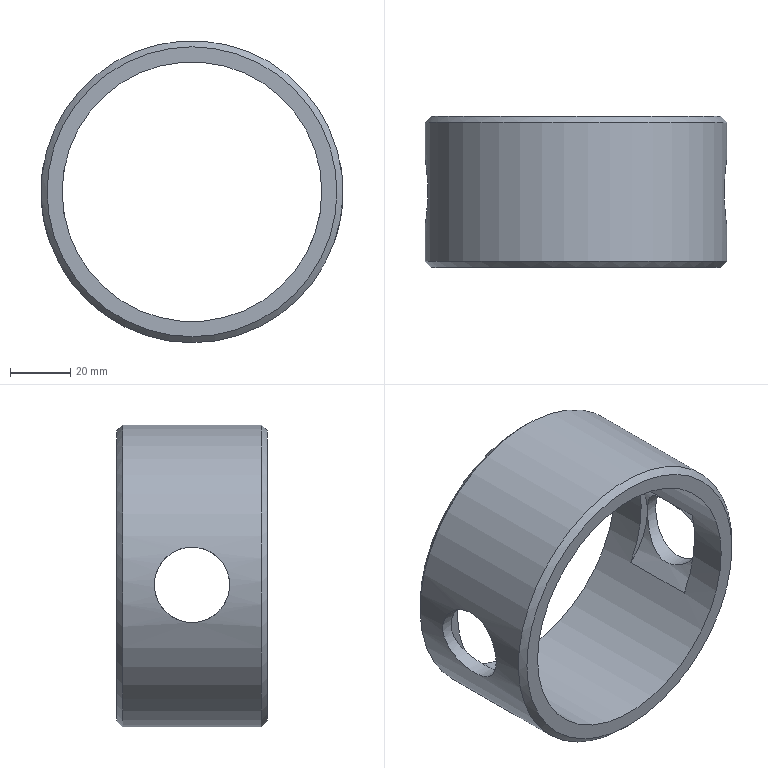Part | NX | features DATUM_CSYS 6, EXTRUDE 5, SKETCH 5, EXTRACT_DATUM_AXIS 4, EXTRACT_DATUM_PLANE 4, EXTRACT_STRING 4, CHAMFER 1, Instance Feature 1, Mirror Feature 1 | 1 solid | 16 faces | box 100.002 x 50 x 100 mm | volume 93333 mm3 | cylinder 8 | plane 6 | cone 2 | commonest cylinder face diameters 44 x4 25 x2 86 x1 100 x1
STEP:
#1=CARTESIAN_POINT('',(-41.856,-12.5,9.851));
#2=VERTEX_POINT('',#1);
#3=CARTESIAN_POINT('',(-46.,-12.5,-3.));
#4=VERTEX_POINT('',#3);
#5=CARTESIAN_POINT('',(-24.,-12.5,-3.));
#6=DIRECTION('',(0.,1.,0.));
#7=DIRECTION('',(-1.,0.,0.));
#8=AXIS2_PLACEMENT_3D('',#5,#6,#7);
#9=CIRCLE('',#8,22.);
#10=EDGE_CURVE('',#2,#4,#9,.F.);
#11=ORIENTED_EDGE('',*,*,#10,.T.);
#12=CARTESIAN_POINT('',(-46.,12.5,-3.));
#13=VERTEX_POINT('',#12);
#14=CARTESIAN_POINT('',(-46.,-12.5,-3.));
#15=CARTESIAN_POINT('',(-46.,-12.5,-1.308));
#16=CARTESIAN_POINT('',(-45.595,-11.807,2.009));
#17=CARTESIAN_POINT('',(-44.159,-9.032,6.076));
#18=CARTESIAN_POINT('',(-42.612,-5.019,8.799));
#19=CARTESIAN_POINT('',(-41.851,-0.003334,9.849));
#20=CARTESIAN_POINT('',(-42.609,5.011,8.804));
#21=CARTESIAN_POINT('',(-44.164,9.044,6.066));
#22=CARTESIAN_POINT('',(-45.595,11.806,2.005));
#23=CARTESIAN_POINT('',(-46.,12.5,-1.306));
#24=CARTESIAN_POINT('',(-46.,12.5,-3.));
#25=B_SPLINE_CURVE_WITH_KNOTS('',3,(#14,#15,#16,#17,#18,#19,#20,#21,#22,#23,#24),.UNSPECIFIED.,.F.,.F.,(4,1,1,1,1,1,1,1,4),(0.,0.004998,0.009995,0.01499,0.01999,0.02499,0.02999,0.03498,0.03998),.UNSPECIFIED.);
#26=EDGE_CURVE('',#13,#4,#25,.F.);
#27=ORIENTED_EDGE('',*,*,#26,.F.);
#28=CARTESIAN_POINT('',(-41.856,12.5,9.851));
#29=VERTEX_POINT('',#28);
#30=CARTESIAN_POINT('',(-24.,12.5,-3.));
#31=DIRECTION('',(0.,1.,0.));
#32=DIRECTION('',(-1.,0.,0.));
#33=AXIS2_PLACEMENT_3D('',#30,#31,#32);
#34=CIRCLE('',#33,22.);
#35=EDGE_CURVE('',#29,#13,#34,.F.);
#36=ORIENTED_EDGE('',*,*,#35,.F.);
#37=CARTESIAN_POINT('',(-41.856,0.,9.851));
#38=DIRECTION('',(0.,1.,0.));
#39=VECTOR('',#38,1000.);
#40=LINE('',#37,#39);
#41=EDGE_CURVE('',#29,#2,#40,.F.);
#42=ORIENTED_EDGE('',*,*,#41,.T.);
#43=EDGE_LOOP('',(#11,#27,#36,#42));
#44=FACE_BOUND('',#43,.T.);
#45=CARTESIAN_POINT('',(-24.,-12.5,-3.));
#46=DIRECTION('',(0.,1.,0.));
#47=DIRECTION('',(0.,0.,1.));
#48=AXIS2_PLACEMENT_3D('',#45,#46,#47);
#49=CYLINDRICAL_SURFACE('',#48,22.);
#50=ADVANCED_FACE('',(#44),#49,.F.);
#51=CARTESIAN_POINT('',(38.144,-12.5,-19.851));
#52=VERTEX_POINT('',#51);
#53=CARTESIAN_POINT('',(41.856,-12.5,9.851));
#54=VERTEX_POINT('',#53);
#55=CARTESIAN_POINT('',(0.,-12.5,0.));
#56=DIRECTION('',(0.,-1.,0.));
#57=DIRECTION('',(0.,0.,-1.));
#58=AXIS2_PLACEMENT_3D('',#55,#56,#57);
#59=CIRCLE('',#58,43.);
#60=EDGE_CURVE('',#52,#54,#59,.T.);
#61=ORIENTED_EDGE('',*,*,#60,.F.);
#62=CARTESIAN_POINT('',(38.144,12.5,-19.851));
#63=VERTEX_POINT('',#62);
#64=CARTESIAN_POINT('',(38.144,0.,-19.851));
#65=DIRECTION('',(0.,1.,0.));
#66=VECTOR('',#65,1000.);
#67=LINE('',#64,#66);
#68=EDGE_CURVE('',#52,#63,#67,.T.);
#69=ORIENTED_EDGE('',*,*,#68,.T.);
#70=CARTESIAN_POINT('',(41.856,12.5,9.851));
#71=VERTEX_POINT('',#70);
#72=CARTESIAN_POINT('',(0.,12.5,0.));
#73=DIRECTION('',(0.,-1.,0.));
#74=DIRECTION('',(0.,0.,-1.));
#75=AXIS2_PLACEMENT_3D('',#72,#73,#74);
#76=CIRCLE('',#75,43.);
#77=EDGE_CURVE('',#63,#71,#76,.T.);
#78=ORIENTED_EDGE('',*,*,#77,.T.);
#79=CARTESIAN_POINT('',(41.856,0.,9.851));
#80=DIRECTION('',(0.,1.,0.));
#81=VECTOR('',#80,1000.);
#82=LINE('',#79,#81);
#83=EDGE_CURVE('',#71,#54,#82,.F.);
#84=ORIENTED_EDGE('',*,*,#83,.T.);
#85=EDGE_LOOP('',(#61,#69,#78,#84));
#86=FACE_BOUND('',#85,.T.);
#87=CARTESIAN_POINT('',(43.,-25.,0.));
#88=VERTEX_POINT('',#87);
#89=CARTESIAN_POINT('',(0.,-25.,0.));
#90=DIRECTION('',(0.,-1.,0.));
#91=DIRECTION('',(1.,0.,0.));
#92=AXIS2_PLACEMENT_3D('',#89,#90,#91);
#93=CIRCLE('',#92,43.);
#94=EDGE_CURVE('',#88,#88,#93,.T.);
#95=ORIENTED_EDGE('',*,*,#94,.T.);
#96=EDGE_LOOP('',(#95));
#97=FACE_BOUND('',#96,.T.);
#98=CARTESIAN_POINT('',(43.,25.,0.));
#99=VERTEX_POINT('',#98);
#100=CARTESIAN_POINT('',(0.,25.,0.));
#101=DIRECTION('',(0.,-1.,0.));
#102=DIRECTION('',(1.,0.,0.));
#103=AXIS2_PLACEMENT_3D('',#100,#101,#102);
#104=CIRCLE('',#103,43.);
#105=EDGE_CURVE('',#99,#99,#104,.T.);
#106=ORIENTED_EDGE('',*,*,#105,.F.);
#107=EDGE_LOOP('',(#106));
#108=FACE_BOUND('',#107,.T.);
#109=CARTESIAN_POINT('',(-38.144,-12.5,-19.851));
#110=VERTEX_POINT('',#109);
#111=CARTESIAN_POINT('',(-38.144,12.5,-19.851));
#112=VERTEX_POINT('',#111);
#113=CARTESIAN_POINT('',(-38.144,0.,-19.851));
#114=DIRECTION('',(0.,1.,0.));
#115=VECTOR('',#114,1000.);
#116=LINE('',#113,#115);
#117=EDGE_CURVE('',#110,#112,#116,.T.);
#118=ORIENTED_EDGE('',*,*,#117,.F.);
#119=CARTESIAN_POINT('',(0.,-12.5,0.));
#120=DIRECTION('',(0.,1.,0.));
#121=DIRECTION('',(0.,0.,1.));
#122=AXIS2_PLACEMENT_3D('',#119,#120,#121);
#123=CIRCLE('',#122,43.);
#124=EDGE_CURVE('',#110,#2,#123,.T.);
#125=ORIENTED_EDGE('',*,*,#124,.T.);
#126=ORIENTED_EDGE('',*,*,#41,.F.);
#127=CARTESIAN_POINT('',(0.,12.5,0.));
#128=DIRECTION('',(0.,1.,0.));
#129=DIRECTION('',(0.,0.,1.));
#130=AXIS2_PLACEMENT_3D('',#127,#128,#129);
#131=CIRCLE('',#130,43.);
#132=EDGE_CURVE('',#112,#29,#131,.T.);
#133=ORIENTED_EDGE('',*,*,#132,.F.);
#134=EDGE_LOOP('',(#118,#125,#126,#133));
#135=FACE_BOUND('',#134,.T.);
#136=CARTESIAN_POINT('',(0.,-25.,0.));
#137=DIRECTION('',(0.,1.,0.));
#138=DIRECTION('',(0.,0.,1.));
#139=AXIS2_PLACEMENT_3D('',#136,#137,#138);
#140=CYLINDRICAL_SURFACE('',#139,43.);
#141=ADVANCED_FACE('',(#86,#97,#108,#135),#140,.F.);
#142=CARTESIAN_POINT('',(-47.537,0.,-15.5));
#143=VERTEX_POINT('',#142);
#144=CARTESIAN_POINT('',(-47.76,-4.945,-14.831));
#145=CARTESIAN_POINT('',(-47.426,0.003336,-15.833));
#146=CARTESIAN_POINT('',(-47.759,4.932,-14.835));
#147=CARTESIAN_POINT('',(-48.841,10.436,-11.16));
#148=CARTESIAN_POINT('',(-49.982,13.155,-4.738));
#149=CARTESIAN_POINT('',(-50.038,11.869,1.862));
#150=CARTESIAN_POINT('',(-49.548,8.172,7.454));
#151=CARTESIAN_POINT('',(-48.784,0.004505,10.863));
#152=CARTESIAN_POINT('',(-49.547,-8.166,7.456));
#153=CARTESIAN_POINT('',(-50.037,-11.861,1.88));
#154=CARTESIAN_POINT('',(-49.983,-13.16,-4.727));
#155=CARTESIAN_POINT('',(-48.841,-10.432,-11.16));
#156=CARTESIAN_POINT('',(-47.76,-4.945,-14.831));
#157=CARTESIAN_POINT('',(-47.426,0.003336,-15.833));
#158=CARTESIAN_POINT('',(-47.759,4.932,-14.835));
#159=B_SPLINE_CURVE_WITH_KNOTS('',3,(#144,#145,#146,#147,#148,#149,#150,#151,#152,#153,#154,#155,#156,#157,#158),.UNSPECIFIED.,.T.,.F.,(1,1,1,1,1,1,1,1,1,1,1,1,1,1,1,1,1,1,1),(-0.01964,-0.009818,-0.004909,0.,0.004909,0.009818,0.01964,0.02454,0.02945,0.03927,0.04909,0.054,0.05891,0.06872,0.07363,0.07854,0.08345,0.08836,0.09818),.UNSPECIFIED.);
#160=EDGE_CURVE('',#143,#143,#159,.T.);
#161=ORIENTED_EDGE('',*,*,#160,.T.);
#162=EDGE_LOOP('',(#161));
#163=FACE_BOUND('',#162,.T.);
#164=CARTESIAN_POINT('',(0.,23.,-50.));
#165=VERTEX_POINT('',#164);
#166=CARTESIAN_POINT('',(0.,23.,0.));
#167=DIRECTION('',(0.,-1.,0.));
#168=DIRECTION('',(0.,0.,-1.));
#169=AXIS2_PLACEMENT_3D('',#166,#167,#168);
#170=CIRCLE('',#169,50.);
#171=EDGE_CURVE('',#165,#165,#170,.T.);
#172=ORIENTED_EDGE('',*,*,#171,.T.);
#173=EDGE_LOOP('',(#172));
#174=FACE_BOUND('',#173,.T.);
#175=CARTESIAN_POINT('',(0.,-23.,-50.));
#176=VERTEX_POINT('',#175);
#177=CARTESIAN_POINT('',(0.,-23.,0.));
#178=DIRECTION('',(0.,-1.,0.));
#179=DIRECTION('',(0.,0.,-1.));
#180=AXIS2_PLACEMENT_3D('',#177,#178,#179);
#181=CIRCLE('',#180,50.);
#182=EDGE_CURVE('',#176,#176,#181,.F.);
#183=ORIENTED_EDGE('',*,*,#182,.T.);
#184=EDGE_LOOP('',(#183));
#185=FACE_BOUND('',#184,.T.);
#186=CARTESIAN_POINT('',(49.089,0.,9.5));
#187=VERTEX_POINT('',#186);
#188=CARTESIAN_POINT('',(49.226,4.95,8.833));
#189=CARTESIAN_POINT('',(48.946,-1.661,10.174));
#190=CARTESIAN_POINT('',(49.547,-8.173,7.448));
#191=CARTESIAN_POINT('',(50.037,-11.863,1.874));
#192=CARTESIAN_POINT('',(49.984,-13.159,-4.717));
#193=CARTESIAN_POINT('',(48.841,-10.434,-11.165));
#194=CARTESIAN_POINT('',(47.758,-4.929,-14.836));
#195=CARTESIAN_POINT('',(47.426,-0.008414,-15.831));
#196=CARTESIAN_POINT('',(47.757,4.918,-14.842));
#197=CARTESIAN_POINT('',(48.839,10.428,-11.172));
#198=CARTESIAN_POINT('',(49.983,13.156,-4.738));
#199=CARTESIAN_POINT('',(50.037,11.87,1.866));
#200=CARTESIAN_POINT('',(49.676,9.094,6.043));
#201=CARTESIAN_POINT('',(49.226,4.95,8.833));
#202=CARTESIAN_POINT('',(48.946,-1.661,10.174));
#203=CARTESIAN_POINT('',(49.547,-8.173,7.448));
#204=B_SPLINE_CURVE_WITH_KNOTS('',3,(#188,#189,#190,#191,#192,#193,#194,#195,#196,#197,#198,#199,#200,#201,#202,#203),.UNSPECIFIED.,.T.,.F.,(1,1,1,1,1,1,1,1,1,1,1,1,1,1,1,1,1,1,1,1),(-0.01473,-0.009817,-0.004909,0.,0.009817,0.01473,0.01963,0.02945,0.03436,0.03927,0.04418,0.04909,0.0589,0.06381,0.06872,0.07363,0.07854,0.08835,0.09326,0.09817),.UNSPECIFIED.);
#205=EDGE_CURVE('',#187,#187,#204,.T.);
#206=ORIENTED_EDGE('',*,*,#205,.F.);
#207=EDGE_LOOP('',(#206));
#208=FACE_BOUND('',#207,.T.);
#209=CARTESIAN_POINT('',(0.,-25.,0.));
#210=DIRECTION('',(0.,1.,0.));
#211=DIRECTION('',(0.,0.,1.));
#212=AXIS2_PLACEMENT_3D('',#209,#210,#211);
#213=CYLINDRICAL_SURFACE('',#212,50.);
#214=ADVANCED_FACE('',(#163,#174,#185,#208),#213,.T.);
#215=CARTESIAN_POINT('',(46.,-12.5,-3.));
#216=VERTEX_POINT('',#215);
#217=CARTESIAN_POINT('',(24.,-12.5,-3.));
#218=DIRECTION('',(0.,-1.,0.));
#219=DIRECTION('',(1.,0.,0.));
#220=AXIS2_PLACEMENT_3D('',#217,#218,#219);
#221=CIRCLE('',#220,22.);
#222=EDGE_CURVE('',#216,#52,#221,.F.);
#223=ORIENTED_EDGE('',*,*,#222,.F.);
#224=CARTESIAN_POINT('',(46.,12.5,-3.));
#225=VERTEX_POINT('',#224);
#226=CARTESIAN_POINT('',(46.,-12.5,-3.));
#227=CARTESIAN_POINT('',(46.,-12.5,-4.692));
#228=CARTESIAN_POINT('',(45.595,-11.807,-8.009));
#229=CARTESIAN_POINT('',(44.159,-9.032,-12.076));
#230=CARTESIAN_POINT('',(42.612,-5.019,-14.799));
#231=CARTESIAN_POINT('',(41.851,-0.003334,-15.849));
#232=CARTESIAN_POINT('',(42.609,5.011,-14.804));
#233=CARTESIAN_POINT('',(44.164,9.044,-12.066));
#234=CARTESIAN_POINT('',(45.595,11.806,-8.005));
#235=CARTESIAN_POINT('',(46.,12.5,-4.694));
#236=CARTESIAN_POINT('',(46.,12.5,-3.));
#237=B_SPLINE_CURVE_WITH_KNOTS('',3,(#226,#227,#228,#229,#230,#231,#232,#233,#234,#235,#236),.UNSPECIFIED.,.F.,.F.,(4,1,1,1,1,1,1,1,4),(0.,0.004998,0.009995,0.01499,0.01999,0.02499,0.02999,0.03498,0.03998),.UNSPECIFIED.);
#238=EDGE_CURVE('',#216,#225,#237,.T.);
#239=ORIENTED_EDGE('',*,*,#238,.T.);
#240=CARTESIAN_POINT('',(24.,12.5,-3.));
#241=DIRECTION('',(0.,-1.,0.));
#242=DIRECTION('',(1.,0.,0.));
#243=AXIS2_PLACEMENT_3D('',#240,#241,#242);
#244=CIRCLE('',#243,22.);
#245=EDGE_CURVE('',#225,#63,#244,.F.);
#246=ORIENTED_EDGE('',*,*,#245,.T.);
#247=ORIENTED_EDGE('',*,*,#68,.F.);
#248=EDGE_LOOP('',(#223,#239,#246,#247));
#249=FACE_BOUND('',#248,.T.);
#250=CARTESIAN_POINT('',(24.,-12.5,-3.));
#251=DIRECTION('',(0.,1.,0.));
#252=DIRECTION('',(0.,0.,1.));
#253=AXIS2_PLACEMENT_3D('',#250,#251,#252);
#254=CYLINDRICAL_SURFACE('',#253,22.);
#255=ADVANCED_FACE('',(#249),#254,.F.);
#256=CARTESIAN_POINT('',(24.,12.5,-3.));
#257=DIRECTION('',(0.,-1.,0.));
#258=DIRECTION('',(1.,0.,0.));
#259=AXIS2_PLACEMENT_3D('',#256,#257,#258);
#260=CIRCLE('',#259,22.);
#261=EDGE_CURVE('',#71,#225,#260,.F.);
#262=ORIENTED_EDGE('',*,*,#261,.T.);
#263=CARTESIAN_POINT('',(46.,12.5,-3.));
#264=CARTESIAN_POINT('',(46.,12.5,-1.31));
#265=CARTESIAN_POINT('',(45.595,11.807,2.009));
#266=CARTESIAN_POINT('',(44.16,9.033,6.074));
#267=CARTESIAN_POINT('',(42.613,5.024,8.797));
#268=CARTESIAN_POINT('',(41.851,0.006648,9.849));
#269=CARTESIAN_POINT('',(42.606,-4.999,8.809));
#270=CARTESIAN_POINT('',(44.16,-9.035,6.072));
#271=CARTESIAN_POINT('',(45.591,-11.798,2.029));
#272=CARTESIAN_POINT('',(46.,-12.5,-1.311));
#273=CARTESIAN_POINT('',(46.,-12.5,-3.));
#274=B_SPLINE_CURVE_WITH_KNOTS('',3,(#263,#264,#265,#266,#267,#268,#269,#270,#271,#272,#273),.UNSPECIFIED.,.F.,.F.,(4,1,1,1,1,1,1,1,4),(0.03998,0.04497,0.04996,0.05494,0.05993,0.06492,0.0699,0.07489,0.07988),.UNSPECIFIED.);
#275=EDGE_CURVE('',#225,#216,#274,.T.);
#276=ORIENTED_EDGE('',*,*,#275,.T.);
#277=CARTESIAN_POINT('',(24.,-12.5,-3.));
#278=DIRECTION('',(0.,-1.,0.));
#279=DIRECTION('',(1.,0.,0.));
#280=AXIS2_PLACEMENT_3D('',#277,#278,#279);
#281=CIRCLE('',#280,22.);
#282=EDGE_CURVE('',#54,#216,#281,.F.);
#283=ORIENTED_EDGE('',*,*,#282,.F.);
#284=ORIENTED_EDGE('',*,*,#83,.F.);
#285=EDGE_LOOP('',(#262,#276,#283,#284));
#286=FACE_BOUND('',#285,.T.);
#287=CARTESIAN_POINT('',(24.,-12.5,-3.));
#288=DIRECTION('',(0.,1.,0.));
#289=DIRECTION('',(0.,0.,1.));
#290=AXIS2_PLACEMENT_3D('',#287,#288,#289);
#291=CYLINDRICAL_SURFACE('',#290,22.);
#292=ADVANCED_FACE('',(#286),#291,.F.);
#293=CARTESIAN_POINT('',(0.,-25.,-48.));
#294=VERTEX_POINT('',#293);
#295=CARTESIAN_POINT('',(0.,-25.,0.));
#296=DIRECTION('',(0.,-1.,0.));
#297=DIRECTION('',(0.,0.,-1.));
#298=AXIS2_PLACEMENT_3D('',#295,#296,#297);
#299=CIRCLE('',#298,48.);
#300=EDGE_CURVE('',#294,#294,#299,.T.);
#301=ORIENTED_EDGE('',*,*,#300,.T.);
#302=EDGE_LOOP('',(#301));
#303=FACE_BOUND('',#302,.T.);
#304=ORIENTED_EDGE('',*,*,#94,.F.);
#305=EDGE_LOOP('',(#304));
#306=FACE_BOUND('',#305,.T.);
#307=CARTESIAN_POINT('',(0.,-25.,0.));
#308=DIRECTION('',(0.,-1.,0.));
#309=DIRECTION('',(0.,0.,-1.));
#310=AXIS2_PLACEMENT_3D('',#307,#308,#309);
#311=PLANE('',#310);
#312=ADVANCED_FACE('',(#303,#306),#311,.T.);
#313=CARTESIAN_POINT('',(0.,25.,-48.));
#314=VERTEX_POINT('',#313);
#315=CARTESIAN_POINT('',(0.,25.,0.));
#316=DIRECTION('',(0.,-1.,0.));
#317=DIRECTION('',(0.,0.,-1.));
#318=AXIS2_PLACEMENT_3D('',#315,#316,#317);
#319=CIRCLE('',#318,48.);
#320=EDGE_CURVE('',#314,#314,#319,.F.);
#321=ORIENTED_EDGE('',*,*,#320,.T.);
#322=EDGE_LOOP('',(#321));
#323=FACE_BOUND('',#322,.T.);
#324=ORIENTED_EDGE('',*,*,#105,.T.);
#325=EDGE_LOOP('',(#324));
#326=FACE_BOUND('',#325,.T.);
#327=CARTESIAN_POINT('',(0.,25.,0.));
#328=DIRECTION('',(0.,-1.,0.));
#329=DIRECTION('',(0.,0.,-1.));
#330=AXIS2_PLACEMENT_3D('',#327,#328,#329);
#331=PLANE('',#330);
#332=ADVANCED_FACE('',(#323,#326),#331,.F.);
#333=ORIENTED_EDGE('',*,*,#320,.F.);
#334=EDGE_LOOP('',(#333));
#335=FACE_BOUND('',#334,.T.);
#336=ORIENTED_EDGE('',*,*,#171,.F.);
#337=EDGE_LOOP('',(#336));
#338=FACE_BOUND('',#337,.T.);
#339=CARTESIAN_POINT('',(0.,23.,0.));
#340=DIRECTION('',(0.,-1.,0.));
#341=DIRECTION('',(0.,0.,-1.));
#342=AXIS2_PLACEMENT_3D('',#339,#340,#341);
#343=CONICAL_SURFACE('',#342,50.,0.7854);
#344=ADVANCED_FACE('',(#335,#338),#343,.T.);
#345=ORIENTED_EDGE('',*,*,#182,.F.);
#346=EDGE_LOOP('',(#345));
#347=FACE_BOUND('',#346,.T.);
#348=ORIENTED_EDGE('',*,*,#300,.F.);
#349=EDGE_LOOP('',(#348));
#350=FACE_BOUND('',#349,.T.);
#351=CARTESIAN_POINT('',(0.,-25.,0.));
#352=DIRECTION('',(0.,1.,0.));
#353=DIRECTION('',(0.,0.,1.));
#354=AXIS2_PLACEMENT_3D('',#351,#352,#353);
#355=CONICAL_SURFACE('',#354,48.,0.7854);
#356=ADVANCED_FACE('',(#347,#350),#355,.T.);
#357=ORIENTED_EDGE('',*,*,#60,.T.);
#358=ORIENTED_EDGE('',*,*,#282,.T.);
#359=ORIENTED_EDGE('',*,*,#222,.T.);
#360=EDGE_LOOP('',(#357,#358,#359));
#361=FACE_BOUND('',#360,.T.);
#362=CARTESIAN_POINT('',(24.,-12.5,-3.));
#363=DIRECTION('',(0.,-1.,0.));
#364=DIRECTION('',(0.,0.,-1.));
#365=AXIS2_PLACEMENT_3D('',#362,#363,#364);
#366=PLANE('',#365);
#367=ADVANCED_FACE('',(#361),#366,.F.);
#368=ORIENTED_EDGE('',*,*,#245,.F.);
#369=ORIENTED_EDGE('',*,*,#261,.F.);
#370=ORIENTED_EDGE('',*,*,#77,.F.);
#371=EDGE_LOOP('',(#368,#369,#370));
#372=FACE_BOUND('',#371,.T.);
#373=CARTESIAN_POINT('',(24.,12.5,-3.));
#374=DIRECTION('',(0.,-1.,0.));
#375=DIRECTION('',(0.,0.,-1.));
#376=AXIS2_PLACEMENT_3D('',#373,#374,#375);
#377=PLANE('',#376);
#378=ADVANCED_FACE('',(#372),#377,.T.);
#379=ORIENTED_EDGE('',*,*,#275,.F.);
#380=ORIENTED_EDGE('',*,*,#238,.F.);
#381=EDGE_LOOP('',(#379,#380));
#382=FACE_BOUND('',#381,.T.);
#383=ORIENTED_EDGE('',*,*,#205,.T.);
#384=EDGE_LOOP('',(#383));
#385=FACE_BOUND('',#384,.T.);
#386=CARTESIAN_POINT('',(55.,0.,-3.));
#387=DIRECTION('',(-1.,0.,0.));
#388=DIRECTION('',(0.,0.,1.));
#389=AXIS2_PLACEMENT_3D('',#386,#387,#388);
#390=CYLINDRICAL_SURFACE('',#389,12.5);
#391=ADVANCED_FACE('',(#382,#385),#390,.F.);
#392=CARTESIAN_POINT('',(-24.,12.5,-3.));
#393=DIRECTION('',(0.,1.,0.));
#394=DIRECTION('',(-1.,0.,0.));
#395=AXIS2_PLACEMENT_3D('',#392,#393,#394);
#396=CIRCLE('',#395,22.);
#397=EDGE_CURVE('',#13,#112,#396,.F.);
#398=ORIENTED_EDGE('',*,*,#397,.F.);
#399=CARTESIAN_POINT('',(-46.,12.5,-3.));
#400=CARTESIAN_POINT('',(-46.,12.5,-4.69));
#401=CARTESIAN_POINT('',(-45.595,11.807,-8.009));
#402=CARTESIAN_POINT('',(-44.16,9.033,-12.074));
#403=CARTESIAN_POINT('',(-42.613,5.024,-14.797));
#404=CARTESIAN_POINT('',(-41.851,0.006648,-15.849));
#405=CARTESIAN_POINT('',(-42.606,-4.999,-14.809));
#406=CARTESIAN_POINT('',(-44.16,-9.035,-12.072));
#407=CARTESIAN_POINT('',(-45.591,-11.798,-8.029));
#408=CARTESIAN_POINT('',(-46.,-12.5,-4.689));
#409=CARTESIAN_POINT('',(-46.,-12.5,-3.));
#410=B_SPLINE_CURVE_WITH_KNOTS('',3,(#399,#400,#401,#402,#403,#404,#405,#406,#407,#408,#409),.UNSPECIFIED.,.F.,.F.,(4,1,1,1,1,1,1,1,4),(0.03998,0.04497,0.04996,0.05494,0.05993,0.06492,0.0699,0.07489,0.07988),.UNSPECIFIED.);
#411=EDGE_CURVE('',#4,#13,#410,.F.);
#412=ORIENTED_EDGE('',*,*,#411,.F.);
#413=CARTESIAN_POINT('',(-24.,-12.5,-3.));
#414=DIRECTION('',(0.,1.,0.));
#415=DIRECTION('',(-1.,0.,0.));
#416=AXIS2_PLACEMENT_3D('',#413,#414,#415);
#417=CIRCLE('',#416,22.);
#418=EDGE_CURVE('',#4,#110,#417,.F.);
#419=ORIENTED_EDGE('',*,*,#418,.T.);
#420=ORIENTED_EDGE('',*,*,#117,.T.);
#421=EDGE_LOOP('',(#398,#412,#419,#420));
#422=FACE_BOUND('',#421,.T.);
#423=CARTESIAN_POINT('',(-24.,-12.5,-3.));
#424=DIRECTION('',(0.,1.,0.));
#425=DIRECTION('',(0.,0.,1.));
#426=AXIS2_PLACEMENT_3D('',#423,#424,#425);
#427=CYLINDRICAL_SURFACE('',#426,22.);
#428=ADVANCED_FACE('',(#422),#427,.F.);
#429=ORIENTED_EDGE('',*,*,#10,.F.);
#430=ORIENTED_EDGE('',*,*,#124,.F.);
#431=ORIENTED_EDGE('',*,*,#418,.F.);
#432=EDGE_LOOP('',(#429,#430,#431));
#433=FACE_BOUND('',#432,.T.);
#434=CARTESIAN_POINT('',(-24.,-12.5,-3.));
#435=DIRECTION('',(0.,1.,0.));
#436=DIRECTION('',(0.,0.,1.));
#437=AXIS2_PLACEMENT_3D('',#434,#435,#436);
#438=PLANE('',#437);
#439=ADVANCED_FACE('',(#433),#438,.T.);
#440=ORIENTED_EDGE('',*,*,#35,.T.);
#441=ORIENTED_EDGE('',*,*,#397,.T.);
#442=ORIENTED_EDGE('',*,*,#132,.T.);
#443=EDGE_LOOP('',(#440,#441,#442));
#444=FACE_BOUND('',#443,.T.);
#445=CARTESIAN_POINT('',(-24.,12.5,-3.));
#446=DIRECTION('',(0.,1.,0.));
#447=DIRECTION('',(0.,0.,1.));
#448=AXIS2_PLACEMENT_3D('',#445,#446,#447);
#449=PLANE('',#448);
#450=ADVANCED_FACE('',(#444),#449,.F.);
#451=ORIENTED_EDGE('',*,*,#411,.T.);
#452=ORIENTED_EDGE('',*,*,#26,.T.);
#453=EDGE_LOOP('',(#451,#452));
#454=FACE_BOUND('',#453,.T.);
#455=ORIENTED_EDGE('',*,*,#160,.F.);
#456=EDGE_LOOP('',(#455));
#457=FACE_BOUND('',#456,.T.);
#458=CARTESIAN_POINT('',(-55.,0.,-3.));
#459=DIRECTION('',(1.,0.,0.));
#460=DIRECTION('',(0.,0.,-1.));
#461=AXIS2_PLACEMENT_3D('',#458,#459,#460);
#462=CYLINDRICAL_SURFACE('',#461,12.5);
#463=ADVANCED_FACE('',(#454,#457),#462,.F.);
#464=CLOSED_SHELL('',(#50,#141,#214,#255,#292,#312,#332,#344,#356,#367,#378,#391,#428,#439,#450,#463));
#465=MANIFOLD_SOLID_BREP('',#464);
#466=(LENGTH_UNIT()NAMED_UNIT(*)SI_UNIT(.MILLI.,.METRE.));
#467=UNCERTAINTY_MEASURE_WITH_UNIT(LENGTH_MEASURE(0.0508),#466,'','');
#468=(NAMED_UNIT(*)PLANE_ANGLE_UNIT()SI_UNIT($,.RADIAN.));
#469=(NAMED_UNIT(*)SI_UNIT($,.STERADIAN.)SOLID_ANGLE_UNIT());
#470=(GEOMETRIC_REPRESENTATION_CONTEXT(3)GLOBAL_UNCERTAINTY_ASSIGNED_CONTEXT((#467))GLOBAL_UNIT_ASSIGNED_CONTEXT((#466,#468,#469))REPRESENTATION_CONTEXT('',''));
#471=ADVANCED_BREP_SHAPE_REPRESENTATION('',(#465),#470);